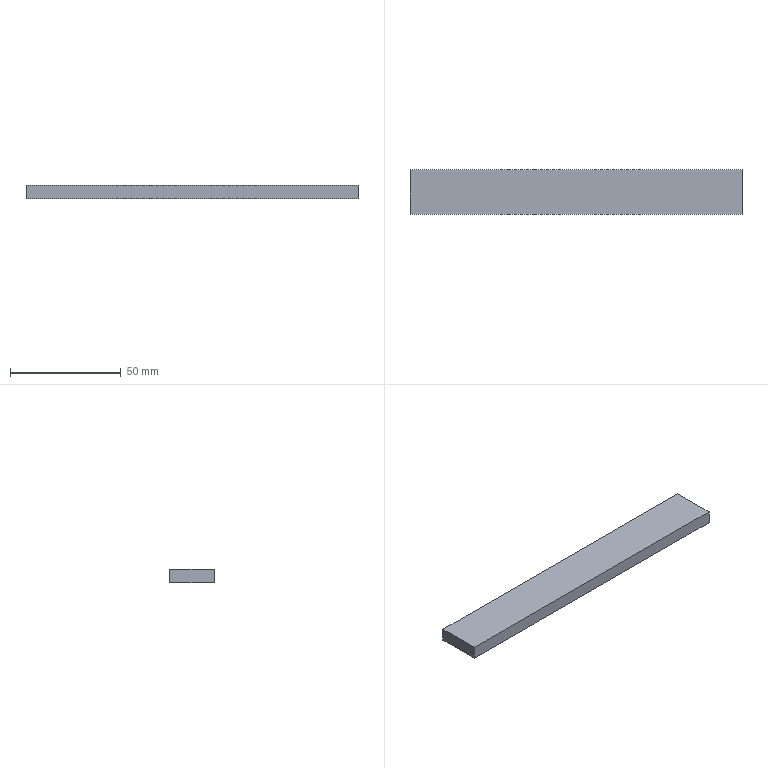Part | SolidWorks | features Extrusion 1 | 1 solid | 6 faces | box 150 x 20 x 6 mm | volume 18000 mm3 | plane 6
STEP:
#1=CARTESIAN_POINT('',(75.,-10.,0.));
#2=VERTEX_POINT('',#1);
#3=CARTESIAN_POINT('',(75.,10.,0.));
#4=VERTEX_POINT('',#3);
#5=CARTESIAN_POINT('',(75.,-10.,0.));
#6=DIRECTION('',(0.,1.,0.));
#7=VECTOR('',#6,1000.);
#8=LINE('',#5,#7);
#9=EDGE_CURVE('',#2,#4,#8,.T.);
#10=ORIENTED_EDGE('',*,*,#9,.T.);
#11=CARTESIAN_POINT('',(75.,10.,6.));
#12=VERTEX_POINT('',#11);
#13=CARTESIAN_POINT('',(75.,10.,6.));
#14=DIRECTION('',(0.,0.,-1.));
#15=VECTOR('',#14,1000.);
#16=LINE('',#13,#15);
#17=EDGE_CURVE('',#12,#4,#16,.T.);
#18=ORIENTED_EDGE('',*,*,#17,.F.);
#19=CARTESIAN_POINT('',(75.,-10.,6.));
#20=VERTEX_POINT('',#19);
#21=CARTESIAN_POINT('',(75.,-10.,6.));
#22=DIRECTION('',(0.,1.,0.));
#23=VECTOR('',#22,1000.);
#24=LINE('',#21,#23);
#25=EDGE_CURVE('',#20,#12,#24,.T.);
#26=ORIENTED_EDGE('',*,*,#25,.F.);
#27=CARTESIAN_POINT('',(75.,-10.,6.));
#28=DIRECTION('',(0.,0.,-1.));
#29=VECTOR('',#28,1000.);
#30=LINE('',#27,#29);
#31=EDGE_CURVE('',#20,#2,#30,.T.);
#32=ORIENTED_EDGE('',*,*,#31,.T.);
#33=EDGE_LOOP('',(#10,#18,#26,#32));
#34=FACE_OUTER_BOUND('',#33,.T.);
#35=CARTESIAN_POINT('',(75.,-10.,6.));
#36=DIRECTION('',(-1.,0.,0.));
#37=DIRECTION('',(0.,0.,1.));
#38=AXIS2_PLACEMENT_3D('',#35,#36,#37);
#39=PLANE('',#38);
#40=ADVANCED_FACE('',(#34),#39,.F.);
#41=CARTESIAN_POINT('',(-75.,10.,0.));
#42=VERTEX_POINT('',#41);
#43=CARTESIAN_POINT('',(-75.,10.,0.));
#44=DIRECTION('',(-1.,0.,0.));
#45=VECTOR('',#44,1000.);
#46=LINE('',#43,#45);
#47=EDGE_CURVE('',#4,#42,#46,.T.);
#48=ORIENTED_EDGE('',*,*,#47,.T.);
#49=CARTESIAN_POINT('',(-75.,10.,6.));
#50=VERTEX_POINT('',#49);
#51=CARTESIAN_POINT('',(-75.,10.,6.));
#52=DIRECTION('',(0.,0.,-1.));
#53=VECTOR('',#52,1000.);
#54=LINE('',#51,#53);
#55=EDGE_CURVE('',#50,#42,#54,.T.);
#56=ORIENTED_EDGE('',*,*,#55,.F.);
#57=CARTESIAN_POINT('',(-75.,10.,6.));
#58=DIRECTION('',(-1.,0.,0.));
#59=VECTOR('',#58,1000.);
#60=LINE('',#57,#59);
#61=EDGE_CURVE('',#12,#50,#60,.T.);
#62=ORIENTED_EDGE('',*,*,#61,.F.);
#63=ORIENTED_EDGE('',*,*,#17,.T.);
#64=EDGE_LOOP('',(#48,#56,#62,#63));
#65=FACE_OUTER_BOUND('',#64,.T.);
#66=CARTESIAN_POINT('',(-75.,10.,6.));
#67=DIRECTION('',(0.,-1.,0.));
#68=DIRECTION('',(0.,0.,-1.));
#69=AXIS2_PLACEMENT_3D('',#66,#67,#68);
#70=PLANE('',#69);
#71=ADVANCED_FACE('',(#65),#70,.F.);
#72=CARTESIAN_POINT('',(-75.,-10.,0.));
#73=VERTEX_POINT('',#72);
#74=CARTESIAN_POINT('',(-75.,-10.,0.));
#75=DIRECTION('',(0.,-1.,0.));
#76=VECTOR('',#75,1000.);
#77=LINE('',#74,#76);
#78=EDGE_CURVE('',#42,#73,#77,.T.);
#79=ORIENTED_EDGE('',*,*,#78,.T.);
#80=CARTESIAN_POINT('',(-75.,-10.,6.));
#81=VERTEX_POINT('',#80);
#82=CARTESIAN_POINT('',(-75.,-10.,6.));
#83=DIRECTION('',(0.,0.,-1.));
#84=VECTOR('',#83,1000.);
#85=LINE('',#82,#84);
#86=EDGE_CURVE('',#81,#73,#85,.T.);
#87=ORIENTED_EDGE('',*,*,#86,.F.);
#88=CARTESIAN_POINT('',(-75.,-10.,6.));
#89=DIRECTION('',(0.,-1.,0.));
#90=VECTOR('',#89,1000.);
#91=LINE('',#88,#90);
#92=EDGE_CURVE('',#50,#81,#91,.T.);
#93=ORIENTED_EDGE('',*,*,#92,.F.);
#94=ORIENTED_EDGE('',*,*,#55,.T.);
#95=EDGE_LOOP('',(#79,#87,#93,#94));
#96=FACE_OUTER_BOUND('',#95,.T.);
#97=CARTESIAN_POINT('',(-75.,-10.,6.));
#98=DIRECTION('',(1.,0.,0.));
#99=DIRECTION('',(0.,0.,-1.));
#100=AXIS2_PLACEMENT_3D('',#97,#98,#99);
#101=PLANE('',#100);
#102=ADVANCED_FACE('',(#96),#101,.F.);
#103=CARTESIAN_POINT('',(-75.,-10.,0.));
#104=DIRECTION('',(1.,0.,0.));
#105=VECTOR('',#104,1000.);
#106=LINE('',#103,#105);
#107=EDGE_CURVE('',#73,#2,#106,.T.);
#108=ORIENTED_EDGE('',*,*,#107,.T.);
#109=ORIENTED_EDGE('',*,*,#31,.F.);
#110=CARTESIAN_POINT('',(-75.,-10.,6.));
#111=DIRECTION('',(1.,0.,0.));
#112=VECTOR('',#111,1000.);
#113=LINE('',#110,#112);
#114=EDGE_CURVE('',#81,#20,#113,.T.);
#115=ORIENTED_EDGE('',*,*,#114,.F.);
#116=ORIENTED_EDGE('',*,*,#86,.T.);
#117=EDGE_LOOP('',(#108,#109,#115,#116));
#118=FACE_OUTER_BOUND('',#117,.T.);
#119=CARTESIAN_POINT('',(-75.,-10.,6.));
#120=DIRECTION('',(0.,1.,0.));
#121=DIRECTION('',(0.,0.,1.));
#122=AXIS2_PLACEMENT_3D('',#119,#120,#121);
#123=PLANE('',#122);
#124=ADVANCED_FACE('',(#118),#123,.F.);
#125=ORIENTED_EDGE('',*,*,#25,.T.);
#126=ORIENTED_EDGE('',*,*,#61,.T.);
#127=ORIENTED_EDGE('',*,*,#92,.T.);
#128=ORIENTED_EDGE('',*,*,#114,.T.);
#129=EDGE_LOOP('',(#125,#126,#127,#128));
#130=FACE_OUTER_BOUND('',#129,.T.);
#131=CARTESIAN_POINT('',(0.,0.,6.));
#132=DIRECTION('',(0.,0.,-1.));
#133=DIRECTION('',(-1.,0.,0.));
#134=AXIS2_PLACEMENT_3D('',#131,#132,#133);
#135=PLANE('',#134);
#136=ADVANCED_FACE('',(#130),#135,.F.);
#137=ORIENTED_EDGE('',*,*,#9,.F.);
#138=ORIENTED_EDGE('',*,*,#107,.F.);
#139=ORIENTED_EDGE('',*,*,#78,.F.);
#140=ORIENTED_EDGE('',*,*,#47,.F.);
#141=EDGE_LOOP('',(#137,#138,#139,#140));
#142=FACE_OUTER_BOUND('',#141,.T.);
#143=CARTESIAN_POINT('',(0.,0.,0.));
#144=DIRECTION('',(0.,0.,-1.));
#145=DIRECTION('',(-1.,0.,0.));
#146=AXIS2_PLACEMENT_3D('',#143,#144,#145);
#147=PLANE('',#146);
#148=ADVANCED_FACE('',(#142),#147,.T.);
#149=CLOSED_SHELL('',(#40,#71,#102,#124,#136,#148));
#150=MANIFOLD_SOLID_BREP('',#149);
#151=CARTESIAN_POINT('',(0.,0.,0.));
#152=DIRECTION('',(0.,0.,1.));
#153=DIRECTION('',(1.,0.,0.));
#154=AXIS2_PLACEMENT_3D('',#151,#152,#153);
#155=(LENGTH_UNIT()NAMED_UNIT(*)SI_UNIT(.MILLI.,.METRE.));
#156=UNCERTAINTY_MEASURE_WITH_UNIT(LENGTH_MEASURE(0.00001),#155,'','');
#157=(NAMED_UNIT(*)PLANE_ANGLE_UNIT()SI_UNIT($,.RADIAN.));
#158=(NAMED_UNIT(*)SI_UNIT($,.STERADIAN.)SOLID_ANGLE_UNIT());
#159=(GEOMETRIC_REPRESENTATION_CONTEXT(3)GLOBAL_UNCERTAINTY_ASSIGNED_CONTEXT((#156))GLOBAL_UNIT_ASSIGNED_CONTEXT((#155,#157,#158))REPRESENTATION_CONTEXT('',''));
#160=ADVANCED_BREP_SHAPE_REPRESENTATION('',(#150,#154),#159);